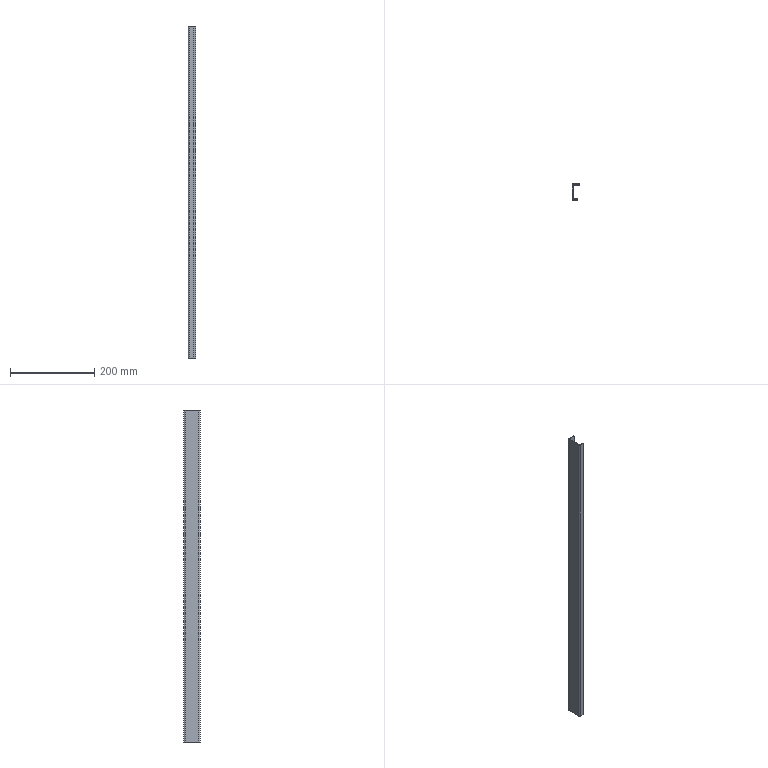Part | STEP file | Electrical Cabinet 4 | 1 solid | 14 faces | box 18 x 38 x 787 mm | volume 98709 mm3 | plane 10 | cylinder 4 | commonest cylinder face diameters 1 x2 5 x2
STEP:
#1=CARTESIAN_POINT('',(59.148,-76.464,787.));
#2=VERTEX_POINT('',#1);
#3=CARTESIAN_POINT('',(59.148,-109.464,787.));
#4=VERTEX_POINT('',#3);
#5=CARTESIAN_POINT('',(59.148,-73.964,787.));
#6=DIRECTION('',(0.,-1.,0.));
#7=VECTOR('',#6,1000.);
#8=LINE('',#5,#7);
#9=EDGE_CURVE('',#2,#4,#8,.T.);
#10=ORIENTED_EDGE('',*,*,#9,.T.);
#11=CARTESIAN_POINT('',(59.148,-109.464,0.));
#12=VERTEX_POINT('',#11);
#13=CARTESIAN_POINT('',(59.148,-109.464,787.));
#14=DIRECTION('',(0.,0.,-1.));
#15=VECTOR('',#14,1000.);
#16=LINE('',#13,#15);
#17=EDGE_CURVE('',#4,#12,#16,.T.);
#18=ORIENTED_EDGE('',*,*,#17,.T.);
#19=CARTESIAN_POINT('',(59.148,-76.464,0.));
#20=VERTEX_POINT('',#19);
#21=CARTESIAN_POINT('',(59.148,-73.964,0.));
#22=DIRECTION('',(0.,1.,0.));
#23=VECTOR('',#22,1000.);
#24=LINE('',#21,#23);
#25=EDGE_CURVE('',#12,#20,#24,.T.);
#26=ORIENTED_EDGE('',*,*,#25,.T.);
#27=CARTESIAN_POINT('',(59.148,-76.464,787.));
#28=DIRECTION('',(0.,0.,1.));
#29=VECTOR('',#28,1000.);
#30=LINE('',#27,#29);
#31=EDGE_CURVE('',#20,#2,#30,.T.);
#32=ORIENTED_EDGE('',*,*,#31,.T.);
#33=EDGE_LOOP('',(#10,#18,#26,#32));
#34=FACE_OUTER_BOUND('',#33,.T.);
#35=CARTESIAN_POINT('',(59.148,-73.964,787.));
#36=DIRECTION('',(1.,0.,0.));
#37=DIRECTION('',(0.,1.,0.));
#38=AXIS2_PLACEMENT_3D('',#35,#36,#37);
#39=PLANE('',#38);
#40=ADVANCED_FACE('',(#34),#39,.T.);
#41=ORIENTED_EDGE('',*,*,#17,.F.);
#42=CARTESIAN_POINT('',(59.648,-109.964,787.));
#43=VERTEX_POINT('',#42);
#44=CARTESIAN_POINT('',(59.648,-109.464,787.));
#45=DIRECTION('',(0.,0.,-1.));
#46=DIRECTION('',(-1.,0.,0.));
#47=AXIS2_PLACEMENT_3D('',#44,#45,#46);
#48=CIRCLE('',#47,0.5);
#49=EDGE_CURVE('',#43,#4,#48,.T.);
#50=ORIENTED_EDGE('',*,*,#49,.F.);
#51=CARTESIAN_POINT('',(59.648,-109.964,0.));
#52=VERTEX_POINT('',#51);
#53=CARTESIAN_POINT('',(59.648,-109.964,787.));
#54=DIRECTION('',(0.,0.,1.));
#55=VECTOR('',#54,1000.);
#56=LINE('',#53,#55);
#57=EDGE_CURVE('',#52,#43,#56,.T.);
#58=ORIENTED_EDGE('',*,*,#57,.F.);
#59=CARTESIAN_POINT('',(59.648,-109.464,0.));
#60=DIRECTION('',(0.,0.,1.));
#61=DIRECTION('',(-1.,0.,0.));
#62=AXIS2_PLACEMENT_3D('',#59,#60,#61);
#63=CIRCLE('',#62,0.5);
#64=EDGE_CURVE('',#12,#52,#63,.T.);
#65=ORIENTED_EDGE('',*,*,#64,.F.);
#66=EDGE_LOOP('',(#41,#50,#58,#65));
#67=FACE_OUTER_BOUND('',#66,.T.);
#68=CARTESIAN_POINT('',(59.648,-109.464,787.));
#69=DIRECTION('',(0.,0.,-1.));
#70=DIRECTION('',(-1.,0.,0.));
#71=AXIS2_PLACEMENT_3D('',#68,#69,#70);
#72=CYLINDRICAL_SURFACE('',#71,0.5);
#73=ADVANCED_FACE('',(#67),#72,.F.);
#74=ORIENTED_EDGE('',*,*,#9,.F.);
#75=CARTESIAN_POINT('',(59.648,-75.964,787.));
#76=VERTEX_POINT('',#75);
#77=CARTESIAN_POINT('',(59.648,-76.464,787.));
#78=DIRECTION('',(0.,0.,-1.));
#79=DIRECTION('',(-1.,0.,0.));
#80=AXIS2_PLACEMENT_3D('',#77,#78,#79);
#81=CIRCLE('',#80,0.5);
#82=EDGE_CURVE('',#2,#76,#81,.T.);
#83=ORIENTED_EDGE('',*,*,#82,.T.);
#84=CARTESIAN_POINT('',(75.148,-75.964,787.));
#85=VERTEX_POINT('',#84);
#86=CARTESIAN_POINT('',(75.148,-75.964,787.));
#87=DIRECTION('',(-1.,0.,0.));
#88=VECTOR('',#87,1000.);
#89=LINE('',#86,#88);
#90=EDGE_CURVE('',#85,#76,#89,.T.);
#91=ORIENTED_EDGE('',*,*,#90,.F.);
#92=CARTESIAN_POINT('',(75.148,-73.964,787.));
#93=VERTEX_POINT('',#92);
#94=CARTESIAN_POINT('',(75.148,-76.464,787.));
#95=DIRECTION('',(0.,1.,0.));
#96=VECTOR('',#95,1000.);
#97=LINE('',#94,#96);
#98=EDGE_CURVE('',#85,#93,#97,.T.);
#99=ORIENTED_EDGE('',*,*,#98,.T.);
#100=CARTESIAN_POINT('',(59.648,-73.964,787.));
#101=VERTEX_POINT('',#100);
#102=CARTESIAN_POINT('',(59.148,-73.964,787.));
#103=DIRECTION('',(-1.,0.,0.));
#104=VECTOR('',#103,1000.);
#105=LINE('',#102,#104);
#106=EDGE_CURVE('',#93,#101,#105,.T.);
#107=ORIENTED_EDGE('',*,*,#106,.T.);
#108=CARTESIAN_POINT('',(57.148,-76.464,787.));
#109=VERTEX_POINT('',#108);
#110=CARTESIAN_POINT('',(59.648,-76.464,787.));
#111=DIRECTION('',(0.,0.,1.));
#112=DIRECTION('',(-1.,0.,0.));
#113=AXIS2_PLACEMENT_3D('',#110,#111,#112);
#114=CIRCLE('',#113,2.5);
#115=EDGE_CURVE('',#101,#109,#114,.T.);
#116=ORIENTED_EDGE('',*,*,#115,.T.);
#117=CARTESIAN_POINT('',(57.148,-109.464,787.));
#118=VERTEX_POINT('',#117);
#119=CARTESIAN_POINT('',(57.148,-109.964,787.));
#120=DIRECTION('',(0.,-1.,0.));
#121=VECTOR('',#120,1000.);
#122=LINE('',#119,#121);
#123=EDGE_CURVE('',#109,#118,#122,.T.);
#124=ORIENTED_EDGE('',*,*,#123,.T.);
#125=CARTESIAN_POINT('',(59.648,-111.964,787.));
#126=VERTEX_POINT('',#125);
#127=CARTESIAN_POINT('',(59.648,-109.464,787.));
#128=DIRECTION('',(0.,0.,1.));
#129=DIRECTION('',(-1.,0.,0.));
#130=AXIS2_PLACEMENT_3D('',#127,#128,#129);
#131=CIRCLE('',#130,2.5);
#132=EDGE_CURVE('',#118,#126,#131,.T.);
#133=ORIENTED_EDGE('',*,*,#132,.T.);
#134=CARTESIAN_POINT('',(69.148,-111.964,787.));
#135=VERTEX_POINT('',#134);
#136=CARTESIAN_POINT('',(59.648,-111.964,787.));
#137=DIRECTION('',(1.,0.,0.));
#138=VECTOR('',#137,1000.);
#139=LINE('',#136,#138);
#140=EDGE_CURVE('',#126,#135,#139,.T.);
#141=ORIENTED_EDGE('',*,*,#140,.T.);
#142=CARTESIAN_POINT('',(69.148,-109.964,787.));
#143=VERTEX_POINT('',#142);
#144=CARTESIAN_POINT('',(69.148,-109.964,787.));
#145=DIRECTION('',(0.,-1.,0.));
#146=VECTOR('',#145,1000.);
#147=LINE('',#144,#146);
#148=EDGE_CURVE('',#143,#135,#147,.T.);
#149=ORIENTED_EDGE('',*,*,#148,.F.);
#150=CARTESIAN_POINT('',(57.148,-109.964,787.));
#151=DIRECTION('',(1.,0.,0.));
#152=VECTOR('',#151,1000.);
#153=LINE('',#150,#152);
#154=EDGE_CURVE('',#43,#143,#153,.T.);
#155=ORIENTED_EDGE('',*,*,#154,.F.);
#156=ORIENTED_EDGE('',*,*,#49,.T.);
#157=EDGE_LOOP('',(#74,#83,#91,#99,#107,#116,#124,#133,#141,#149,#155,#156));
#158=FACE_OUTER_BOUND('',#157,.T.);
#159=CARTESIAN_POINT('',(59.648,-109.964,787.));
#160=DIRECTION('',(0.,0.,1.));
#161=DIRECTION('',(1.,0.,0.));
#162=AXIS2_PLACEMENT_3D('',#159,#160,#161);
#163=PLANE('',#162);
#164=ADVANCED_FACE('',(#158),#163,.T.);
#165=CARTESIAN_POINT('',(59.648,-75.964,0.));
#166=VERTEX_POINT('',#165);
#167=CARTESIAN_POINT('',(59.648,-75.964,787.));
#168=DIRECTION('',(0.,0.,-1.));
#169=VECTOR('',#168,1000.);
#170=LINE('',#167,#169);
#171=EDGE_CURVE('',#76,#166,#170,.T.);
#172=ORIENTED_EDGE('',*,*,#171,.F.);
#173=ORIENTED_EDGE('',*,*,#82,.F.);
#174=ORIENTED_EDGE('',*,*,#31,.F.);
#175=CARTESIAN_POINT('',(59.648,-76.464,0.));
#176=DIRECTION('',(0.,0.,1.));
#177=DIRECTION('',(-1.,0.,0.));
#178=AXIS2_PLACEMENT_3D('',#175,#176,#177);
#179=CIRCLE('',#178,0.5);
#180=EDGE_CURVE('',#166,#20,#179,.T.);
#181=ORIENTED_EDGE('',*,*,#180,.F.);
#182=EDGE_LOOP('',(#172,#173,#174,#181));
#183=FACE_OUTER_BOUND('',#182,.T.);
#184=CARTESIAN_POINT('',(59.648,-76.464,787.));
#185=DIRECTION('',(0.,0.,-1.));
#186=DIRECTION('',(-1.,0.,0.));
#187=AXIS2_PLACEMENT_3D('',#184,#185,#186);
#188=CYLINDRICAL_SURFACE('',#187,0.5);
#189=ADVANCED_FACE('',(#183),#188,.F.);
#190=ORIENTED_EDGE('',*,*,#25,.F.);
#191=ORIENTED_EDGE('',*,*,#64,.T.);
#192=CARTESIAN_POINT('',(69.148,-109.964,0.));
#193=VERTEX_POINT('',#192);
#194=CARTESIAN_POINT('',(57.148,-109.964,0.));
#195=DIRECTION('',(-1.,0.,0.));
#196=VECTOR('',#195,1000.);
#197=LINE('',#194,#196);
#198=EDGE_CURVE('',#193,#52,#197,.T.);
#199=ORIENTED_EDGE('',*,*,#198,.F.);
#200=CARTESIAN_POINT('',(69.148,-111.964,0.));
#201=VERTEX_POINT('',#200);
#202=CARTESIAN_POINT('',(69.148,-109.964,0.));
#203=DIRECTION('',(0.,1.,0.));
#204=VECTOR('',#203,1000.);
#205=LINE('',#202,#204);
#206=EDGE_CURVE('',#201,#193,#205,.T.);
#207=ORIENTED_EDGE('',*,*,#206,.F.);
#208=CARTESIAN_POINT('',(59.648,-111.964,0.));
#209=VERTEX_POINT('',#208);
#210=CARTESIAN_POINT('',(59.148,-111.964,0.));
#211=DIRECTION('',(-1.,0.,0.));
#212=VECTOR('',#211,1000.);
#213=LINE('',#210,#212);
#214=EDGE_CURVE('',#201,#209,#213,.T.);
#215=ORIENTED_EDGE('',*,*,#214,.T.);
#216=CARTESIAN_POINT('',(57.148,-109.464,0.));
#217=VERTEX_POINT('',#216);
#218=CARTESIAN_POINT('',(59.648,-109.464,0.));
#219=DIRECTION('',(0.,0.,-1.));
#220=DIRECTION('',(-1.,0.,0.));
#221=AXIS2_PLACEMENT_3D('',#218,#219,#220);
#222=CIRCLE('',#221,2.5);
#223=EDGE_CURVE('',#209,#217,#222,.T.);
#224=ORIENTED_EDGE('',*,*,#223,.T.);
#225=CARTESIAN_POINT('',(57.148,-76.464,0.));
#226=VERTEX_POINT('',#225);
#227=CARTESIAN_POINT('',(57.148,-75.964,0.));
#228=DIRECTION('',(0.,1.,0.));
#229=VECTOR('',#228,1000.);
#230=LINE('',#227,#229);
#231=EDGE_CURVE('',#217,#226,#230,.T.);
#232=ORIENTED_EDGE('',*,*,#231,.T.);
#233=CARTESIAN_POINT('',(59.648,-73.964,0.));
#234=VERTEX_POINT('',#233);
#235=CARTESIAN_POINT('',(59.648,-76.464,0.));
#236=DIRECTION('',(0.,0.,-1.));
#237=DIRECTION('',(-1.,0.,0.));
#238=AXIS2_PLACEMENT_3D('',#235,#236,#237);
#239=CIRCLE('',#238,2.5);
#240=EDGE_CURVE('',#226,#234,#239,.T.);
#241=ORIENTED_EDGE('',*,*,#240,.T.);
#242=CARTESIAN_POINT('',(75.148,-73.964,0.));
#243=VERTEX_POINT('',#242);
#244=CARTESIAN_POINT('',(59.648,-73.964,0.));
#245=DIRECTION('',(-1.,0.,0.));
#246=VECTOR('',#245,1000.);
#247=LINE('',#244,#246);
#248=EDGE_CURVE('',#243,#234,#247,.T.);
#249=ORIENTED_EDGE('',*,*,#248,.F.);
#250=CARTESIAN_POINT('',(75.148,-75.964,0.));
#251=VERTEX_POINT('',#250);
#252=CARTESIAN_POINT('',(75.148,-73.964,0.));
#253=DIRECTION('',(0.,1.,0.));
#254=VECTOR('',#253,1000.);
#255=LINE('',#252,#254);
#256=EDGE_CURVE('',#251,#243,#255,.T.);
#257=ORIENTED_EDGE('',*,*,#256,.F.);
#258=CARTESIAN_POINT('',(75.148,-75.964,0.));
#259=DIRECTION('',(1.,0.,0.));
#260=VECTOR('',#259,1000.);
#261=LINE('',#258,#260);
#262=EDGE_CURVE('',#166,#251,#261,.T.);
#263=ORIENTED_EDGE('',*,*,#262,.F.);
#264=ORIENTED_EDGE('',*,*,#180,.T.);
#265=EDGE_LOOP('',(#190,#191,#199,#207,#215,#224,#232,#241,#249,#257,#263,#264));
#266=FACE_OUTER_BOUND('',#265,.T.);
#267=CARTESIAN_POINT('',(59.648,-75.964,0.));
#268=DIRECTION('',(0.,0.,-1.));
#269=DIRECTION('',(-1.,0.,0.));
#270=AXIS2_PLACEMENT_3D('',#267,#268,#269);
#271=PLANE('',#270);
#272=ADVANCED_FACE('',(#266),#271,.T.);
#273=ORIENTED_EDGE('',*,*,#154,.T.);
#274=CARTESIAN_POINT('',(69.148,-109.964,787.));
#275=DIRECTION('',(0.,0.,-1.));
#276=VECTOR('',#275,1000.);
#277=LINE('',#274,#276);
#278=EDGE_CURVE('',#143,#193,#277,.T.);
#279=ORIENTED_EDGE('',*,*,#278,.T.);
#280=ORIENTED_EDGE('',*,*,#198,.T.);
#281=ORIENTED_EDGE('',*,*,#57,.T.);
#282=EDGE_LOOP('',(#273,#279,#280,#281));
#283=FACE_OUTER_BOUND('',#282,.T.);
#284=CARTESIAN_POINT('',(57.148,-109.964,787.));
#285=DIRECTION('',(0.,1.,0.));
#286=DIRECTION('',(0.,0.,1.));
#287=AXIS2_PLACEMENT_3D('',#284,#285,#286);
#288=PLANE('',#287);
#289=ADVANCED_FACE('',(#283),#288,.T.);
#290=CARTESIAN_POINT('',(57.148,-109.464,787.));
#291=DIRECTION('',(0.,0.,-1.));
#292=VECTOR('',#291,1000.);
#293=LINE('',#290,#292);
#294=EDGE_CURVE('',#118,#217,#293,.T.);
#295=ORIENTED_EDGE('',*,*,#294,.F.);
#296=ORIENTED_EDGE('',*,*,#123,.F.);
#297=CARTESIAN_POINT('',(57.148,-76.464,787.));
#298=DIRECTION('',(0.,0.,1.));
#299=VECTOR('',#298,1000.);
#300=LINE('',#297,#299);
#301=EDGE_CURVE('',#226,#109,#300,.T.);
#302=ORIENTED_EDGE('',*,*,#301,.F.);
#303=ORIENTED_EDGE('',*,*,#231,.F.);
#304=EDGE_LOOP('',(#295,#296,#302,#303));
#305=FACE_OUTER_BOUND('',#304,.T.);
#306=CARTESIAN_POINT('',(57.148,-73.964,787.));
#307=DIRECTION('',(1.,0.,0.));
#308=DIRECTION('',(0.,1.,0.));
#309=AXIS2_PLACEMENT_3D('',#306,#307,#308);
#310=PLANE('',#309);
#311=ADVANCED_FACE('',(#305),#310,.F.);
#312=ORIENTED_EDGE('',*,*,#90,.T.);
#313=ORIENTED_EDGE('',*,*,#171,.T.);
#314=ORIENTED_EDGE('',*,*,#262,.T.);
#315=CARTESIAN_POINT('',(75.148,-75.964,787.));
#316=DIRECTION('',(0.,0.,1.));
#317=VECTOR('',#316,1000.);
#318=LINE('',#315,#317);
#319=EDGE_CURVE('',#251,#85,#318,.T.);
#320=ORIENTED_EDGE('',*,*,#319,.T.);
#321=EDGE_LOOP('',(#312,#313,#314,#320));
#322=FACE_OUTER_BOUND('',#321,.T.);
#323=CARTESIAN_POINT('',(75.148,-75.964,787.));
#324=DIRECTION('',(0.,-1.,0.));
#325=DIRECTION('',(0.,0.,-1.));
#326=AXIS2_PLACEMENT_3D('',#323,#324,#325);
#327=PLANE('',#326);
#328=ADVANCED_FACE('',(#322),#327,.T.);
#329=ORIENTED_EDGE('',*,*,#148,.T.);
#330=CARTESIAN_POINT('',(69.148,-111.964,787.));
#331=DIRECTION('',(0.,0.,-1.));
#332=VECTOR('',#331,1000.);
#333=LINE('',#330,#332);
#334=EDGE_CURVE('',#135,#201,#333,.T.);
#335=ORIENTED_EDGE('',*,*,#334,.T.);
#336=ORIENTED_EDGE('',*,*,#206,.T.);
#337=ORIENTED_EDGE('',*,*,#278,.F.);
#338=EDGE_LOOP('',(#329,#335,#336,#337));
#339=FACE_OUTER_BOUND('',#338,.T.);
#340=CARTESIAN_POINT('',(69.148,-109.964,787.));
#341=DIRECTION('',(1.,0.,0.));
#342=DIRECTION('',(0.,0.,-1.));
#343=AXIS2_PLACEMENT_3D('',#340,#341,#342);
#344=PLANE('',#343);
#345=ADVANCED_FACE('',(#339),#344,.T.);
#346=ORIENTED_EDGE('',*,*,#115,.F.);
#347=CARTESIAN_POINT('',(59.648,-73.964,787.));
#348=DIRECTION('',(0.,0.,-1.));
#349=VECTOR('',#348,1000.);
#350=LINE('',#347,#349);
#351=EDGE_CURVE('',#101,#234,#350,.T.);
#352=ORIENTED_EDGE('',*,*,#351,.T.);
#353=ORIENTED_EDGE('',*,*,#240,.F.);
#354=ORIENTED_EDGE('',*,*,#301,.T.);
#355=EDGE_LOOP('',(#346,#352,#353,#354));
#356=FACE_OUTER_BOUND('',#355,.T.);
#357=CARTESIAN_POINT('',(59.648,-76.464,787.));
#358=DIRECTION('',(0.,0.,-1.));
#359=DIRECTION('',(-1.,0.,0.));
#360=AXIS2_PLACEMENT_3D('',#357,#358,#359);
#361=CYLINDRICAL_SURFACE('',#360,2.5);
#362=ADVANCED_FACE('',(#356),#361,.T.);
#363=ORIENTED_EDGE('',*,*,#132,.F.);
#364=ORIENTED_EDGE('',*,*,#294,.T.);
#365=ORIENTED_EDGE('',*,*,#223,.F.);
#366=CARTESIAN_POINT('',(59.648,-111.964,787.));
#367=DIRECTION('',(0.,0.,1.));
#368=VECTOR('',#367,1000.);
#369=LINE('',#366,#368);
#370=EDGE_CURVE('',#209,#126,#369,.T.);
#371=ORIENTED_EDGE('',*,*,#370,.T.);
#372=EDGE_LOOP('',(#363,#364,#365,#371));
#373=FACE_OUTER_BOUND('',#372,.T.);
#374=CARTESIAN_POINT('',(59.648,-109.464,787.));
#375=DIRECTION('',(0.,0.,-1.));
#376=DIRECTION('',(-1.,0.,0.));
#377=AXIS2_PLACEMENT_3D('',#374,#375,#376);
#378=CYLINDRICAL_SURFACE('',#377,2.5);
#379=ADVANCED_FACE('',(#373),#378,.T.);
#380=ORIENTED_EDGE('',*,*,#98,.F.);
#381=ORIENTED_EDGE('',*,*,#319,.F.);
#382=ORIENTED_EDGE('',*,*,#256,.T.);
#383=CARTESIAN_POINT('',(75.148,-73.964,787.));
#384=DIRECTION('',(0.,0.,1.));
#385=VECTOR('',#384,1000.);
#386=LINE('',#383,#385);
#387=EDGE_CURVE('',#243,#93,#386,.T.);
#388=ORIENTED_EDGE('',*,*,#387,.T.);
#389=EDGE_LOOP('',(#380,#381,#382,#388));
#390=FACE_OUTER_BOUND('',#389,.T.);
#391=CARTESIAN_POINT('',(75.148,-73.964,787.));
#392=DIRECTION('',(1.,0.,0.));
#393=DIRECTION('',(0.,0.,-1.));
#394=AXIS2_PLACEMENT_3D('',#391,#392,#393);
#395=PLANE('',#394);
#396=ADVANCED_FACE('',(#390),#395,.T.);
#397=ORIENTED_EDGE('',*,*,#334,.F.);
#398=ORIENTED_EDGE('',*,*,#140,.F.);
#399=ORIENTED_EDGE('',*,*,#370,.F.);
#400=ORIENTED_EDGE('',*,*,#214,.F.);
#401=EDGE_LOOP('',(#397,#398,#399,#400));
#402=FACE_OUTER_BOUND('',#401,.T.);
#403=CARTESIAN_POINT('',(57.148,-111.964,787.));
#404=DIRECTION('',(0.,1.,0.));
#405=DIRECTION('',(0.,0.,1.));
#406=AXIS2_PLACEMENT_3D('',#403,#404,#405);
#407=PLANE('',#406);
#408=ADVANCED_FACE('',(#402),#407,.F.);
#409=ORIENTED_EDGE('',*,*,#351,.F.);
#410=ORIENTED_EDGE('',*,*,#106,.F.);
#411=ORIENTED_EDGE('',*,*,#387,.F.);
#412=ORIENTED_EDGE('',*,*,#248,.T.);
#413=EDGE_LOOP('',(#409,#410,#411,#412));
#414=FACE_OUTER_BOUND('',#413,.T.);
#415=CARTESIAN_POINT('',(75.148,-73.964,787.));
#416=DIRECTION('',(0.,-1.,0.));
#417=DIRECTION('',(0.,0.,-1.));
#418=AXIS2_PLACEMENT_3D('',#415,#416,#417);
#419=PLANE('',#418);
#420=ADVANCED_FACE('',(#414),#419,.F.);
#421=CLOSED_SHELL('',(#40,#73,#164,#189,#272,#289,#311,#328,#345,#362,#379,#396,#408,#420));
#422=MANIFOLD_SOLID_BREP('',#421);
#423=CARTESIAN_POINT('',(0.,0.,0.));
#424=DIRECTION('',(0.,0.,1.));
#425=DIRECTION('',(1.,0.,0.));
#426=AXIS2_PLACEMENT_3D('',#423,#424,#425);
#427=(LENGTH_UNIT()NAMED_UNIT(*)SI_UNIT(.MILLI.,.METRE.));
#428=UNCERTAINTY_MEASURE_WITH_UNIT(LENGTH_MEASURE(0.00001),#427,'','');
#429=(NAMED_UNIT(*)PLANE_ANGLE_UNIT()SI_UNIT($,.RADIAN.));
#430=(NAMED_UNIT(*)SI_UNIT($,.STERADIAN.)SOLID_ANGLE_UNIT());
#431=(GEOMETRIC_REPRESENTATION_CONTEXT(3)GLOBAL_UNCERTAINTY_ASSIGNED_CONTEXT((#428))GLOBAL_UNIT_ASSIGNED_CONTEXT((#427,#429,#430))REPRESENTATION_CONTEXT('',''));
#432=ADVANCED_BREP_SHAPE_REPRESENTATION('',(#422,#426),#431);